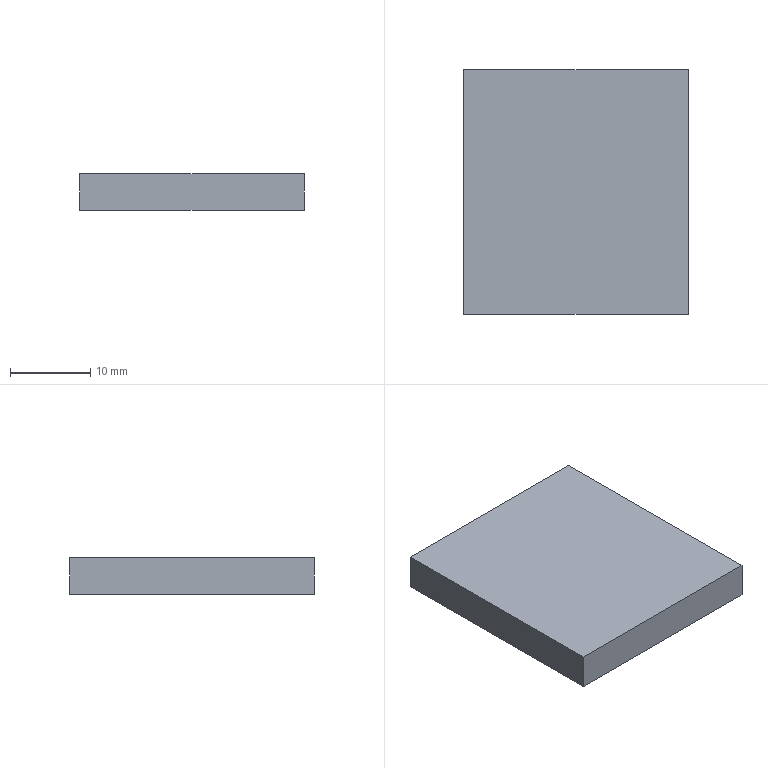Part | SolidWorks | features FlatPattern 1, SMBaseFlange 1, SheetMetal 1 | 1 solid | 6 faces | box 28 x 30.5 x 4.5 mm | volume 3843 mm3 | plane 6
STEP:
#1=CARTESIAN_POINT('',(18011.71,-96157.421,0.));
#2=VERTEX_POINT('',#1);
#3=CARTESIAN_POINT('',(18011.71,-96126.921,0.));
#4=VERTEX_POINT('',#3);
#5=CARTESIAN_POINT('',(18011.71,-96157.421,0.));
#6=DIRECTION('',(0.,1.,0.));
#7=VECTOR('',#6,1000.);
#8=LINE('',#5,#7);
#9=EDGE_CURVE('',#2,#4,#8,.T.);
#10=ORIENTED_EDGE('',*,*,#9,.F.);
#11=CARTESIAN_POINT('',(18011.71,-96157.421,-4.5));
#12=VERTEX_POINT('',#11);
#13=CARTESIAN_POINT('',(18011.71,-96157.421,-4.5));
#14=DIRECTION('',(0.,0.,1.));
#15=VECTOR('',#14,1000.);
#16=LINE('',#13,#15);
#17=EDGE_CURVE('',#12,#2,#16,.T.);
#18=ORIENTED_EDGE('',*,*,#17,.F.);
#19=CARTESIAN_POINT('',(18011.71,-96126.921,-4.5));
#20=VERTEX_POINT('',#19);
#21=CARTESIAN_POINT('',(18011.71,-96157.421,-4.5));
#22=DIRECTION('',(0.,1.,0.));
#23=VECTOR('',#22,1000.);
#24=LINE('',#21,#23);
#25=EDGE_CURVE('',#12,#20,#24,.T.);
#26=ORIENTED_EDGE('',*,*,#25,.T.);
#27=CARTESIAN_POINT('',(18011.71,-96126.921,-4.5));
#28=DIRECTION('',(0.,0.,1.));
#29=VECTOR('',#28,1000.);
#30=LINE('',#27,#29);
#31=EDGE_CURVE('',#20,#4,#30,.T.);
#32=ORIENTED_EDGE('',*,*,#31,.T.);
#33=EDGE_LOOP('',(#10,#18,#26,#32));
#34=FACE_OUTER_BOUND('',#33,.T.);
#35=CARTESIAN_POINT('',(18011.71,-96157.421,-4.5));
#36=DIRECTION('',(1.,0.,0.));
#37=DIRECTION('',(0.,0.,-1.));
#38=AXIS2_PLACEMENT_3D('',#35,#36,#37);
#39=PLANE('',#38);
#40=ADVANCED_FACE('',(#34),#39,.T.);
#41=CARTESIAN_POINT('',(17983.71,-96157.421,0.));
#42=VERTEX_POINT('',#41);
#43=CARTESIAN_POINT('',(17983.71,-96157.421,0.));
#44=DIRECTION('',(1.,0.,0.));
#45=VECTOR('',#44,1000.);
#46=LINE('',#43,#45);
#47=EDGE_CURVE('',#42,#2,#46,.T.);
#48=ORIENTED_EDGE('',*,*,#47,.F.);
#49=CARTESIAN_POINT('',(17983.71,-96157.421,-4.5));
#50=VERTEX_POINT('',#49);
#51=CARTESIAN_POINT('',(17983.71,-96157.421,-4.5));
#52=DIRECTION('',(0.,0.,1.));
#53=VECTOR('',#52,1000.);
#54=LINE('',#51,#53);
#55=EDGE_CURVE('',#50,#42,#54,.T.);
#56=ORIENTED_EDGE('',*,*,#55,.F.);
#57=CARTESIAN_POINT('',(17983.71,-96157.421,-4.5));
#58=DIRECTION('',(1.,0.,0.));
#59=VECTOR('',#58,1000.);
#60=LINE('',#57,#59);
#61=EDGE_CURVE('',#50,#12,#60,.T.);
#62=ORIENTED_EDGE('',*,*,#61,.T.);
#63=ORIENTED_EDGE('',*,*,#17,.T.);
#64=EDGE_LOOP('',(#48,#56,#62,#63));
#65=FACE_OUTER_BOUND('',#64,.T.);
#66=CARTESIAN_POINT('',(17983.71,-96157.421,-4.5));
#67=DIRECTION('',(0.,-1.,0.));
#68=DIRECTION('',(1.,0.,0.));
#69=AXIS2_PLACEMENT_3D('',#66,#67,#68);
#70=PLANE('',#69);
#71=ADVANCED_FACE('',(#65),#70,.T.);
#72=CARTESIAN_POINT('',(17983.71,-96126.921,0.));
#73=VERTEX_POINT('',#72);
#74=CARTESIAN_POINT('',(17983.71,-96132.421,0.));
#75=DIRECTION('',(0.,-1.,0.));
#76=VECTOR('',#75,1000.);
#77=LINE('',#74,#76);
#78=EDGE_CURVE('',#73,#42,#77,.T.);
#79=ORIENTED_EDGE('',*,*,#78,.F.);
#80=CARTESIAN_POINT('',(17983.71,-96126.921,-4.5));
#81=VERTEX_POINT('',#80);
#82=CARTESIAN_POINT('',(17983.71,-96126.921,-4.5));
#83=DIRECTION('',(0.,0.,1.));
#84=VECTOR('',#83,1000.);
#85=LINE('',#82,#84);
#86=EDGE_CURVE('',#81,#73,#85,.T.);
#87=ORIENTED_EDGE('',*,*,#86,.F.);
#88=CARTESIAN_POINT('',(17983.71,-96126.921,-4.5));
#89=DIRECTION('',(0.,-1.,0.));
#90=VECTOR('',#89,1000.);
#91=LINE('',#88,#90);
#92=EDGE_CURVE('',#81,#50,#91,.T.);
#93=ORIENTED_EDGE('',*,*,#92,.T.);
#94=ORIENTED_EDGE('',*,*,#55,.T.);
#95=EDGE_LOOP('',(#79,#87,#93,#94));
#96=FACE_OUTER_BOUND('',#95,.T.);
#97=CARTESIAN_POINT('',(17983.71,-96132.421,-4.5));
#98=DIRECTION('',(-1.,0.,0.));
#99=DIRECTION('',(0.,0.,1.));
#100=AXIS2_PLACEMENT_3D('',#97,#98,#99);
#101=PLANE('',#100);
#102=ADVANCED_FACE('',(#96),#101,.T.);
#103=CARTESIAN_POINT('',(18011.71,-96126.921,0.));
#104=DIRECTION('',(-1.,0.,0.));
#105=VECTOR('',#104,1000.);
#106=LINE('',#103,#105);
#107=EDGE_CURVE('',#4,#73,#106,.T.);
#108=ORIENTED_EDGE('',*,*,#107,.F.);
#109=ORIENTED_EDGE('',*,*,#31,.F.);
#110=CARTESIAN_POINT('',(18011.71,-96126.921,-4.5));
#111=DIRECTION('',(-1.,0.,0.));
#112=VECTOR('',#111,1000.);
#113=LINE('',#110,#112);
#114=EDGE_CURVE('',#20,#81,#113,.T.);
#115=ORIENTED_EDGE('',*,*,#114,.T.);
#116=ORIENTED_EDGE('',*,*,#86,.T.);
#117=EDGE_LOOP('',(#108,#109,#115,#116));
#118=FACE_OUTER_BOUND('',#117,.T.);
#119=CARTESIAN_POINT('',(18011.71,-96126.921,-4.5));
#120=DIRECTION('',(0.,1.,0.));
#121=DIRECTION('',(-1.,0.,0.));
#122=AXIS2_PLACEMENT_3D('',#119,#120,#121);
#123=PLANE('',#122);
#124=ADVANCED_FACE('',(#118),#123,.T.);
#125=ORIENTED_EDGE('',*,*,#25,.F.);
#126=ORIENTED_EDGE('',*,*,#61,.F.);
#127=ORIENTED_EDGE('',*,*,#92,.F.);
#128=ORIENTED_EDGE('',*,*,#114,.F.);
#129=EDGE_LOOP('',(#125,#126,#127,#128));
#130=FACE_OUTER_BOUND('',#129,.T.);
#131=CARTESIAN_POINT('',(0.,0.,-4.5));
#132=DIRECTION('',(0.,0.,1.));
#133=DIRECTION('',(1.,0.,0.));
#134=AXIS2_PLACEMENT_3D('',#131,#132,#133);
#135=PLANE('',#134);
#136=ADVANCED_FACE('',(#130),#135,.F.);
#137=ORIENTED_EDGE('',*,*,#9,.T.);
#138=ORIENTED_EDGE('',*,*,#107,.T.);
#139=ORIENTED_EDGE('',*,*,#78,.T.);
#140=ORIENTED_EDGE('',*,*,#47,.T.);
#141=EDGE_LOOP('',(#137,#138,#139,#140));
#142=FACE_OUTER_BOUND('',#141,.T.);
#143=CARTESIAN_POINT('',(0.,0.,0.));
#144=DIRECTION('',(0.,0.,1.));
#145=DIRECTION('',(1.,0.,0.));
#146=AXIS2_PLACEMENT_3D('',#143,#144,#145);
#147=PLANE('',#146);
#148=ADVANCED_FACE('',(#142),#147,.T.);
#149=CLOSED_SHELL('',(#40,#71,#102,#124,#136,#148));
#150=MANIFOLD_SOLID_BREP('',#149);
#151=CARTESIAN_POINT('',(0.,0.,0.));
#152=DIRECTION('',(0.,0.,1.));
#153=DIRECTION('',(1.,0.,0.));
#154=AXIS2_PLACEMENT_3D('',#151,#152,#153);
#155=(LENGTH_UNIT()NAMED_UNIT(*)SI_UNIT(.MILLI.,.METRE.));
#156=UNCERTAINTY_MEASURE_WITH_UNIT(LENGTH_MEASURE(0.00001),#155,'','');
#157=(NAMED_UNIT(*)PLANE_ANGLE_UNIT()SI_UNIT($,.RADIAN.));
#158=(NAMED_UNIT(*)SI_UNIT($,.STERADIAN.)SOLID_ANGLE_UNIT());
#159=(GEOMETRIC_REPRESENTATION_CONTEXT(3)GLOBAL_UNCERTAINTY_ASSIGNED_CONTEXT((#156))GLOBAL_UNIT_ASSIGNED_CONTEXT((#155,#157,#158))REPRESENTATION_CONTEXT('',''));
#160=ADVANCED_BREP_SHAPE_REPRESENTATION('',(#150,#154),#159);